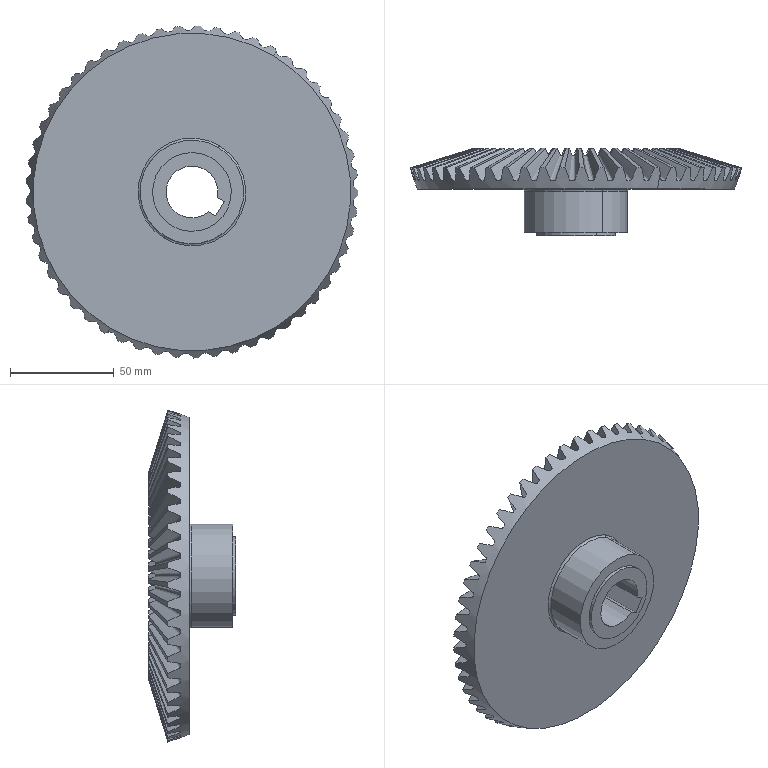Part | SolidWorks | features BaseBody 1 | 1 solid | 126 faces | box 160.088 x 42.208 x 160.125 mm | volume 285045 mm3 | cone 57 | spline 53 | cylinder 7 | plane 7 | torus 2 | commonest cylinder face diameters 25 x3 38 x2 50 x2